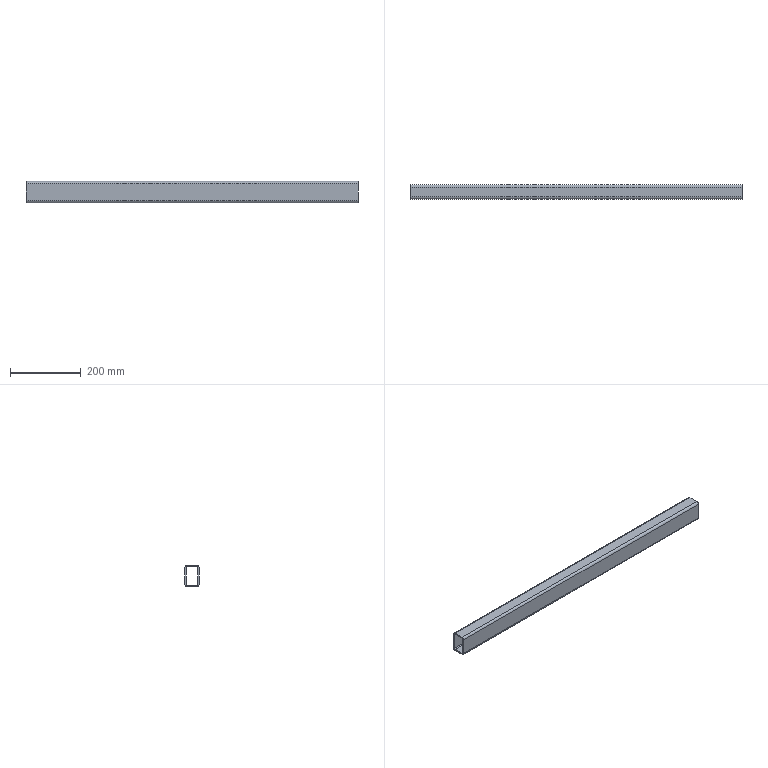Part | STEP file | 40 x 60 x 940_Default<Machined> | 1 solid | 18 faces | box 940 x 40 x 60 mm | volume 663437 mm3 | plane 10 | cylinder 8 | commonest cylinder face diameters 4.8 x4 12.8 x4
STEP:
#1=CARTESIAN_POINT('',(-587.922,20.,23.6));
#2=VERTEX_POINT('',#1);
#3=CARTESIAN_POINT('',(-587.922,13.6,30.));
#4=VERTEX_POINT('',#3);
#5=CARTESIAN_POINT('',(-587.922,13.6,23.6));
#6=DIRECTION('',(1.,0.,0.));
#7=DIRECTION('',(0.,0.,-1.));
#8=AXIS2_PLACEMENT_3D('',#5,#6,#7);
#9=CIRCLE('',#8,6.4);
#10=EDGE_CURVE('',#2,#4,#9,.T.);
#11=ORIENTED_EDGE('',*,*,#10,.T.);
#12=CARTESIAN_POINT('',(352.078,13.6,30.));
#13=VERTEX_POINT('',#12);
#14=CARTESIAN_POINT('',(352.078,13.6,30.));
#15=DIRECTION('',(-1.,0.,0.));
#16=VECTOR('',#15,1000.);
#17=LINE('',#14,#16);
#18=EDGE_CURVE('',#13,#4,#17,.T.);
#19=ORIENTED_EDGE('',*,*,#18,.F.);
#20=CARTESIAN_POINT('',(352.078,20.,23.6));
#21=VERTEX_POINT('',#20);
#22=CARTESIAN_POINT('',(352.078,13.6,23.6));
#23=DIRECTION('',(1.,0.,0.));
#24=DIRECTION('',(0.,0.,-1.));
#25=AXIS2_PLACEMENT_3D('',#22,#23,#24);
#26=CIRCLE('',#25,6.4);
#27=EDGE_CURVE('',#21,#13,#26,.T.);
#28=ORIENTED_EDGE('',*,*,#27,.F.);
#29=CARTESIAN_POINT('',(352.078,20.,23.6));
#30=DIRECTION('',(-1.,0.,0.));
#31=VECTOR('',#30,1000.);
#32=LINE('',#29,#31);
#33=EDGE_CURVE('',#21,#2,#32,.T.);
#34=ORIENTED_EDGE('',*,*,#33,.T.);
#35=EDGE_LOOP('',(#11,#19,#28,#34));
#36=FACE_OUTER_BOUND('',#35,.T.);
#37=CARTESIAN_POINT('',(352.078,13.6,23.6));
#38=DIRECTION('',(-1.,0.,0.));
#39=DIRECTION('',(0.,0.,1.));
#40=AXIS2_PLACEMENT_3D('',#37,#38,#39);
#41=CYLINDRICAL_SURFACE('',#40,6.4);
#42=ADVANCED_FACE('',(#36),#41,.T.);
#43=CARTESIAN_POINT('',(-587.922,-13.6,30.));
#44=VERTEX_POINT('',#43);
#45=CARTESIAN_POINT('',(-587.922,13.6,30.));
#46=DIRECTION('',(0.,-1.,0.));
#47=VECTOR('',#46,1000.);
#48=LINE('',#45,#47);
#49=EDGE_CURVE('',#4,#44,#48,.T.);
#50=ORIENTED_EDGE('',*,*,#49,.T.);
#51=CARTESIAN_POINT('',(352.078,-13.6,30.));
#52=VERTEX_POINT('',#51);
#53=CARTESIAN_POINT('',(352.078,-13.6,30.));
#54=DIRECTION('',(-1.,0.,0.));
#55=VECTOR('',#54,1000.);
#56=LINE('',#53,#55);
#57=EDGE_CURVE('',#52,#44,#56,.T.);
#58=ORIENTED_EDGE('',*,*,#57,.F.);
#59=CARTESIAN_POINT('',(352.078,13.6,30.));
#60=DIRECTION('',(0.,-1.,0.));
#61=VECTOR('',#60,1000.);
#62=LINE('',#59,#61);
#63=EDGE_CURVE('',#13,#52,#62,.T.);
#64=ORIENTED_EDGE('',*,*,#63,.F.);
#65=ORIENTED_EDGE('',*,*,#18,.T.);
#66=EDGE_LOOP('',(#50,#58,#64,#65));
#67=FACE_OUTER_BOUND('',#66,.T.);
#68=CARTESIAN_POINT('',(352.078,13.6,30.));
#69=DIRECTION('',(0.,0.,-1.));
#70=DIRECTION('',(-1.,0.,0.));
#71=AXIS2_PLACEMENT_3D('',#68,#69,#70);
#72=PLANE('',#71);
#73=ADVANCED_FACE('',(#67),#72,.F.);
#74=CARTESIAN_POINT('',(-587.922,-20.,23.6));
#75=VERTEX_POINT('',#74);
#76=CARTESIAN_POINT('',(-587.922,-13.6,23.6));
#77=DIRECTION('',(1.,0.,0.));
#78=DIRECTION('',(0.,0.,-1.));
#79=AXIS2_PLACEMENT_3D('',#76,#77,#78);
#80=CIRCLE('',#79,6.4);
#81=EDGE_CURVE('',#44,#75,#80,.T.);
#82=ORIENTED_EDGE('',*,*,#81,.T.);
#83=CARTESIAN_POINT('',(352.078,-20.,23.6));
#84=VERTEX_POINT('',#83);
#85=CARTESIAN_POINT('',(352.078,-20.,23.6));
#86=DIRECTION('',(-1.,0.,0.));
#87=VECTOR('',#86,1000.);
#88=LINE('',#85,#87);
#89=EDGE_CURVE('',#84,#75,#88,.T.);
#90=ORIENTED_EDGE('',*,*,#89,.F.);
#91=CARTESIAN_POINT('',(352.078,-13.6,23.6));
#92=DIRECTION('',(1.,0.,0.));
#93=DIRECTION('',(0.,0.,-1.));
#94=AXIS2_PLACEMENT_3D('',#91,#92,#93);
#95=CIRCLE('',#94,6.4);
#96=EDGE_CURVE('',#52,#84,#95,.T.);
#97=ORIENTED_EDGE('',*,*,#96,.F.);
#98=ORIENTED_EDGE('',*,*,#57,.T.);
#99=EDGE_LOOP('',(#82,#90,#97,#98));
#100=FACE_OUTER_BOUND('',#99,.T.);
#101=CARTESIAN_POINT('',(352.078,-13.6,23.6));
#102=DIRECTION('',(-1.,0.,0.));
#103=DIRECTION('',(0.,0.,1.));
#104=AXIS2_PLACEMENT_3D('',#101,#102,#103);
#105=CYLINDRICAL_SURFACE('',#104,6.4);
#106=ADVANCED_FACE('',(#100),#105,.T.);
#107=CARTESIAN_POINT('',(-587.922,-20.,-23.6));
#108=VERTEX_POINT('',#107);
#109=CARTESIAN_POINT('',(-587.922,-20.,-23.6));
#110=DIRECTION('',(0.,0.,-1.));
#111=VECTOR('',#110,1000.);
#112=LINE('',#109,#111);
#113=EDGE_CURVE('',#75,#108,#112,.T.);
#114=ORIENTED_EDGE('',*,*,#113,.T.);
#115=CARTESIAN_POINT('',(352.078,-20.,-23.6));
#116=VERTEX_POINT('',#115);
#117=CARTESIAN_POINT('',(352.078,-20.,-23.6));
#118=DIRECTION('',(-1.,0.,0.));
#119=VECTOR('',#118,1000.);
#120=LINE('',#117,#119);
#121=EDGE_CURVE('',#116,#108,#120,.T.);
#122=ORIENTED_EDGE('',*,*,#121,.F.);
#123=CARTESIAN_POINT('',(352.078,-20.,-23.6));
#124=DIRECTION('',(0.,0.,-1.));
#125=VECTOR('',#124,1000.);
#126=LINE('',#123,#125);
#127=EDGE_CURVE('',#84,#116,#126,.T.);
#128=ORIENTED_EDGE('',*,*,#127,.F.);
#129=ORIENTED_EDGE('',*,*,#89,.T.);
#130=EDGE_LOOP('',(#114,#122,#128,#129));
#131=FACE_OUTER_BOUND('',#130,.T.);
#132=CARTESIAN_POINT('',(352.078,-20.,-23.6));
#133=DIRECTION('',(0.,1.,0.));
#134=DIRECTION('',(0.,0.,1.));
#135=AXIS2_PLACEMENT_3D('',#132,#133,#134);
#136=PLANE('',#135);
#137=ADVANCED_FACE('',(#131),#136,.F.);
#138=CARTESIAN_POINT('',(-587.922,-13.6,-30.));
#139=VERTEX_POINT('',#138);
#140=CARTESIAN_POINT('',(-587.922,-13.6,-23.6));
#141=DIRECTION('',(1.,0.,0.));
#142=DIRECTION('',(0.,0.,-1.));
#143=AXIS2_PLACEMENT_3D('',#140,#141,#142);
#144=CIRCLE('',#143,6.4);
#145=EDGE_CURVE('',#108,#139,#144,.T.);
#146=ORIENTED_EDGE('',*,*,#145,.T.);
#147=CARTESIAN_POINT('',(352.078,-13.6,-30.));
#148=VERTEX_POINT('',#147);
#149=CARTESIAN_POINT('',(352.078,-13.6,-30.));
#150=DIRECTION('',(-1.,0.,0.));
#151=VECTOR('',#150,1000.);
#152=LINE('',#149,#151);
#153=EDGE_CURVE('',#148,#139,#152,.T.);
#154=ORIENTED_EDGE('',*,*,#153,.F.);
#155=CARTESIAN_POINT('',(352.078,-13.6,-23.6));
#156=DIRECTION('',(1.,0.,0.));
#157=DIRECTION('',(0.,0.,-1.));
#158=AXIS2_PLACEMENT_3D('',#155,#156,#157);
#159=CIRCLE('',#158,6.4);
#160=EDGE_CURVE('',#116,#148,#159,.T.);
#161=ORIENTED_EDGE('',*,*,#160,.F.);
#162=ORIENTED_EDGE('',*,*,#121,.T.);
#163=EDGE_LOOP('',(#146,#154,#161,#162));
#164=FACE_OUTER_BOUND('',#163,.T.);
#165=CARTESIAN_POINT('',(352.078,-13.6,-23.6));
#166=DIRECTION('',(-1.,0.,0.));
#167=DIRECTION('',(0.,0.,1.));
#168=AXIS2_PLACEMENT_3D('',#165,#166,#167);
#169=CYLINDRICAL_SURFACE('',#168,6.4);
#170=ADVANCED_FACE('',(#164),#169,.T.);
#171=CARTESIAN_POINT('',(-587.922,13.6,-30.));
#172=VERTEX_POINT('',#171);
#173=CARTESIAN_POINT('',(-587.922,-13.6,-30.));
#174=DIRECTION('',(0.,1.,0.));
#175=VECTOR('',#174,1000.);
#176=LINE('',#173,#175);
#177=EDGE_CURVE('',#139,#172,#176,.T.);
#178=ORIENTED_EDGE('',*,*,#177,.T.);
#179=CARTESIAN_POINT('',(352.078,13.6,-30.));
#180=VERTEX_POINT('',#179);
#181=CARTESIAN_POINT('',(352.078,13.6,-30.));
#182=DIRECTION('',(-1.,0.,0.));
#183=VECTOR('',#182,1000.);
#184=LINE('',#181,#183);
#185=EDGE_CURVE('',#180,#172,#184,.T.);
#186=ORIENTED_EDGE('',*,*,#185,.F.);
#187=CARTESIAN_POINT('',(352.078,-13.6,-30.));
#188=DIRECTION('',(0.,1.,0.));
#189=VECTOR('',#188,1000.);
#190=LINE('',#187,#189);
#191=EDGE_CURVE('',#148,#180,#190,.T.);
#192=ORIENTED_EDGE('',*,*,#191,.F.);
#193=ORIENTED_EDGE('',*,*,#153,.T.);
#194=EDGE_LOOP('',(#178,#186,#192,#193));
#195=FACE_OUTER_BOUND('',#194,.T.);
#196=CARTESIAN_POINT('',(352.078,-13.6,-30.));
#197=DIRECTION('',(0.,0.,1.));
#198=DIRECTION('',(1.,0.,0.));
#199=AXIS2_PLACEMENT_3D('',#196,#197,#198);
#200=PLANE('',#199);
#201=ADVANCED_FACE('',(#195),#200,.F.);
#202=CARTESIAN_POINT('',(-587.922,20.,-23.6));
#203=VERTEX_POINT('',#202);
#204=CARTESIAN_POINT('',(-587.922,13.6,-23.6));
#205=DIRECTION('',(1.,0.,0.));
#206=DIRECTION('',(0.,0.,-1.));
#207=AXIS2_PLACEMENT_3D('',#204,#205,#206);
#208=CIRCLE('',#207,6.4);
#209=EDGE_CURVE('',#172,#203,#208,.T.);
#210=ORIENTED_EDGE('',*,*,#209,.T.);
#211=CARTESIAN_POINT('',(352.078,20.,-23.6));
#212=VERTEX_POINT('',#211);
#213=CARTESIAN_POINT('',(352.078,20.,-23.6));
#214=DIRECTION('',(-1.,0.,0.));
#215=VECTOR('',#214,1000.);
#216=LINE('',#213,#215);
#217=EDGE_CURVE('',#212,#203,#216,.T.);
#218=ORIENTED_EDGE('',*,*,#217,.F.);
#219=CARTESIAN_POINT('',(352.078,13.6,-23.6));
#220=DIRECTION('',(1.,0.,0.));
#221=DIRECTION('',(0.,0.,-1.));
#222=AXIS2_PLACEMENT_3D('',#219,#220,#221);
#223=CIRCLE('',#222,6.4);
#224=EDGE_CURVE('',#180,#212,#223,.T.);
#225=ORIENTED_EDGE('',*,*,#224,.F.);
#226=ORIENTED_EDGE('',*,*,#185,.T.);
#227=EDGE_LOOP('',(#210,#218,#225,#226));
#228=FACE_OUTER_BOUND('',#227,.T.);
#229=CARTESIAN_POINT('',(352.078,13.6,-23.6));
#230=DIRECTION('',(-1.,0.,0.));
#231=DIRECTION('',(0.,0.,1.));
#232=AXIS2_PLACEMENT_3D('',#229,#230,#231);
#233=CYLINDRICAL_SURFACE('',#232,6.4);
#234=ADVANCED_FACE('',(#228),#233,.T.);
#235=CARTESIAN_POINT('',(-587.922,-13.6,26.));
#236=VERTEX_POINT('',#235);
#237=CARTESIAN_POINT('',(-587.922,-16.,23.6));
#238=VERTEX_POINT('',#237);
#239=CARTESIAN_POINT('',(-587.922,-13.6,23.6));
#240=DIRECTION('',(1.,0.,0.));
#241=DIRECTION('',(0.,0.,-1.));
#242=AXIS2_PLACEMENT_3D('',#239,#240,#241);
#243=CIRCLE('',#242,2.4);
#244=EDGE_CURVE('',#236,#238,#243,.T.);
#245=ORIENTED_EDGE('',*,*,#244,.F.);
#246=CARTESIAN_POINT('',(352.078,-13.6,26.));
#247=VERTEX_POINT('',#246);
#248=CARTESIAN_POINT('',(352.078,-13.6,26.));
#249=DIRECTION('',(-1.,0.,0.));
#250=VECTOR('',#249,1000.);
#251=LINE('',#248,#250);
#252=EDGE_CURVE('',#247,#236,#251,.T.);
#253=ORIENTED_EDGE('',*,*,#252,.F.);
#254=CARTESIAN_POINT('',(352.078,-16.,23.6));
#255=VERTEX_POINT('',#254);
#256=CARTESIAN_POINT('',(352.078,-13.6,23.6));
#257=DIRECTION('',(1.,0.,0.));
#258=DIRECTION('',(0.,0.,-1.));
#259=AXIS2_PLACEMENT_3D('',#256,#257,#258);
#260=CIRCLE('',#259,2.4);
#261=EDGE_CURVE('',#247,#255,#260,.T.);
#262=ORIENTED_EDGE('',*,*,#261,.T.);
#263=CARTESIAN_POINT('',(352.078,-16.,23.6));
#264=DIRECTION('',(-1.,0.,0.));
#265=VECTOR('',#264,1000.);
#266=LINE('',#263,#265);
#267=EDGE_CURVE('',#255,#238,#266,.T.);
#268=ORIENTED_EDGE('',*,*,#267,.T.);
#269=EDGE_LOOP('',(#245,#253,#262,#268));
#270=FACE_OUTER_BOUND('',#269,.T.);
#271=CARTESIAN_POINT('',(352.078,-13.6,23.6));
#272=DIRECTION('',(-1.,0.,0.));
#273=DIRECTION('',(0.,0.,1.));
#274=AXIS2_PLACEMENT_3D('',#271,#272,#273);
#275=CYLINDRICAL_SURFACE('',#274,2.4);
#276=ADVANCED_FACE('',(#270),#275,.F.);
#277=CARTESIAN_POINT('',(-587.922,13.6,26.));
#278=VERTEX_POINT('',#277);
#279=CARTESIAN_POINT('',(-587.922,13.6,26.));
#280=DIRECTION('',(0.,-1.,0.));
#281=VECTOR('',#280,1000.);
#282=LINE('',#279,#281);
#283=EDGE_CURVE('',#278,#236,#282,.T.);
#284=ORIENTED_EDGE('',*,*,#283,.F.);
#285=CARTESIAN_POINT('',(352.078,13.6,26.));
#286=VERTEX_POINT('',#285);
#287=CARTESIAN_POINT('',(352.078,13.6,26.));
#288=DIRECTION('',(-1.,0.,0.));
#289=VECTOR('',#288,1000.);
#290=LINE('',#287,#289);
#291=EDGE_CURVE('',#286,#278,#290,.T.);
#292=ORIENTED_EDGE('',*,*,#291,.F.);
#293=CARTESIAN_POINT('',(352.078,13.6,26.));
#294=DIRECTION('',(0.,-1.,0.));
#295=VECTOR('',#294,1000.);
#296=LINE('',#293,#295);
#297=EDGE_CURVE('',#286,#247,#296,.T.);
#298=ORIENTED_EDGE('',*,*,#297,.T.);
#299=ORIENTED_EDGE('',*,*,#252,.T.);
#300=EDGE_LOOP('',(#284,#292,#298,#299));
#301=FACE_OUTER_BOUND('',#300,.T.);
#302=CARTESIAN_POINT('',(352.078,13.6,26.));
#303=DIRECTION('',(0.,0.,-1.));
#304=DIRECTION('',(-1.,0.,0.));
#305=AXIS2_PLACEMENT_3D('',#302,#303,#304);
#306=PLANE('',#305);
#307=ADVANCED_FACE('',(#301),#306,.T.);
#308=CARTESIAN_POINT('',(-587.922,16.,23.6));
#309=VERTEX_POINT('',#308);
#310=CARTESIAN_POINT('',(-587.922,13.6,23.6));
#311=DIRECTION('',(1.,0.,0.));
#312=DIRECTION('',(0.,0.,-1.));
#313=AXIS2_PLACEMENT_3D('',#310,#311,#312);
#314=CIRCLE('',#313,2.4);
#315=EDGE_CURVE('',#309,#278,#314,.T.);
#316=ORIENTED_EDGE('',*,*,#315,.F.);
#317=CARTESIAN_POINT('',(352.078,16.,23.6));
#318=VERTEX_POINT('',#317);
#319=CARTESIAN_POINT('',(352.078,16.,23.6));
#320=DIRECTION('',(-1.,0.,0.));
#321=VECTOR('',#320,1000.);
#322=LINE('',#319,#321);
#323=EDGE_CURVE('',#318,#309,#322,.T.);
#324=ORIENTED_EDGE('',*,*,#323,.F.);
#325=CARTESIAN_POINT('',(352.078,13.6,23.6));
#326=DIRECTION('',(1.,0.,0.));
#327=DIRECTION('',(0.,0.,-1.));
#328=AXIS2_PLACEMENT_3D('',#325,#326,#327);
#329=CIRCLE('',#328,2.4);
#330=EDGE_CURVE('',#318,#286,#329,.T.);
#331=ORIENTED_EDGE('',*,*,#330,.T.);
#332=ORIENTED_EDGE('',*,*,#291,.T.);
#333=EDGE_LOOP('',(#316,#324,#331,#332));
#334=FACE_OUTER_BOUND('',#333,.T.);
#335=CARTESIAN_POINT('',(352.078,13.6,23.6));
#336=DIRECTION('',(-1.,0.,0.));
#337=DIRECTION('',(0.,0.,1.));
#338=AXIS2_PLACEMENT_3D('',#335,#336,#337);
#339=CYLINDRICAL_SURFACE('',#338,2.4);
#340=ADVANCED_FACE('',(#334),#339,.F.);
#341=CARTESIAN_POINT('',(-587.922,16.,-23.6));
#342=VERTEX_POINT('',#341);
#343=CARTESIAN_POINT('',(-587.922,16.,23.6));
#344=DIRECTION('',(0.,0.,1.));
#345=VECTOR('',#344,1000.);
#346=LINE('',#343,#345);
#347=EDGE_CURVE('',#342,#309,#346,.T.);
#348=ORIENTED_EDGE('',*,*,#347,.F.);
#349=CARTESIAN_POINT('',(352.078,16.,-23.6));
#350=VERTEX_POINT('',#349);
#351=CARTESIAN_POINT('',(352.078,16.,-23.6));
#352=DIRECTION('',(-1.,0.,0.));
#353=VECTOR('',#352,1000.);
#354=LINE('',#351,#353);
#355=EDGE_CURVE('',#350,#342,#354,.T.);
#356=ORIENTED_EDGE('',*,*,#355,.F.);
#357=CARTESIAN_POINT('',(352.078,16.,23.6));
#358=DIRECTION('',(0.,0.,1.));
#359=VECTOR('',#358,1000.);
#360=LINE('',#357,#359);
#361=EDGE_CURVE('',#350,#318,#360,.T.);
#362=ORIENTED_EDGE('',*,*,#361,.T.);
#363=ORIENTED_EDGE('',*,*,#323,.T.);
#364=EDGE_LOOP('',(#348,#356,#362,#363));
#365=FACE_OUTER_BOUND('',#364,.T.);
#366=CARTESIAN_POINT('',(352.078,16.,23.6));
#367=DIRECTION('',(0.,-1.,0.));
#368=DIRECTION('',(0.,0.,-1.));
#369=AXIS2_PLACEMENT_3D('',#366,#367,#368);
#370=PLANE('',#369);
#371=ADVANCED_FACE('',(#365),#370,.T.);
#372=CARTESIAN_POINT('',(-587.922,13.6,-26.));
#373=VERTEX_POINT('',#372);
#374=CARTESIAN_POINT('',(-587.922,13.6,-23.6));
#375=DIRECTION('',(1.,0.,0.));
#376=DIRECTION('',(0.,0.,-1.));
#377=AXIS2_PLACEMENT_3D('',#374,#375,#376);
#378=CIRCLE('',#377,2.4);
#379=EDGE_CURVE('',#373,#342,#378,.T.);
#380=ORIENTED_EDGE('',*,*,#379,.F.);
#381=CARTESIAN_POINT('',(352.078,13.6,-26.));
#382=VERTEX_POINT('',#381);
#383=CARTESIAN_POINT('',(352.078,13.6,-26.));
#384=DIRECTION('',(-1.,0.,0.));
#385=VECTOR('',#384,1000.);
#386=LINE('',#383,#385);
#387=EDGE_CURVE('',#382,#373,#386,.T.);
#388=ORIENTED_EDGE('',*,*,#387,.F.);
#389=CARTESIAN_POINT('',(352.078,13.6,-23.6));
#390=DIRECTION('',(1.,0.,0.));
#391=DIRECTION('',(0.,0.,-1.));
#392=AXIS2_PLACEMENT_3D('',#389,#390,#391);
#393=CIRCLE('',#392,2.4);
#394=EDGE_CURVE('',#382,#350,#393,.T.);
#395=ORIENTED_EDGE('',*,*,#394,.T.);
#396=ORIENTED_EDGE('',*,*,#355,.T.);
#397=EDGE_LOOP('',(#380,#388,#395,#396));
#398=FACE_OUTER_BOUND('',#397,.T.);
#399=CARTESIAN_POINT('',(352.078,13.6,-23.6));
#400=DIRECTION('',(-1.,0.,0.));
#401=DIRECTION('',(0.,0.,1.));
#402=AXIS2_PLACEMENT_3D('',#399,#400,#401);
#403=CYLINDRICAL_SURFACE('',#402,2.4);
#404=ADVANCED_FACE('',(#398),#403,.F.);
#405=CARTESIAN_POINT('',(-587.922,-13.6,-26.));
#406=VERTEX_POINT('',#405);
#407=CARTESIAN_POINT('',(-587.922,-13.6,-26.));
#408=DIRECTION('',(0.,1.,0.));
#409=VECTOR('',#408,1000.);
#410=LINE('',#407,#409);
#411=EDGE_CURVE('',#406,#373,#410,.T.);
#412=ORIENTED_EDGE('',*,*,#411,.F.);
#413=CARTESIAN_POINT('',(352.078,-13.6,-26.));
#414=VERTEX_POINT('',#413);
#415=CARTESIAN_POINT('',(352.078,-13.6,-26.));
#416=DIRECTION('',(-1.,0.,0.));
#417=VECTOR('',#416,1000.);
#418=LINE('',#415,#417);
#419=EDGE_CURVE('',#414,#406,#418,.T.);
#420=ORIENTED_EDGE('',*,*,#419,.F.);
#421=CARTESIAN_POINT('',(352.078,-13.6,-26.));
#422=DIRECTION('',(0.,1.,0.));
#423=VECTOR('',#422,1000.);
#424=LINE('',#421,#423);
#425=EDGE_CURVE('',#414,#382,#424,.T.);
#426=ORIENTED_EDGE('',*,*,#425,.T.);
#427=ORIENTED_EDGE('',*,*,#387,.T.);
#428=EDGE_LOOP('',(#412,#420,#426,#427));
#429=FACE_OUTER_BOUND('',#428,.T.);
#430=CARTESIAN_POINT('',(352.078,-13.6,-26.));
#431=DIRECTION('',(0.,0.,1.));
#432=DIRECTION('',(1.,0.,0.));
#433=AXIS2_PLACEMENT_3D('',#430,#431,#432);
#434=PLANE('',#433);
#435=ADVANCED_FACE('',(#429),#434,.T.);
#436=CARTESIAN_POINT('',(-587.922,-16.,-23.6));
#437=VERTEX_POINT('',#436);
#438=CARTESIAN_POINT('',(-587.922,-13.6,-23.6));
#439=DIRECTION('',(1.,0.,0.));
#440=DIRECTION('',(0.,0.,-1.));
#441=AXIS2_PLACEMENT_3D('',#438,#439,#440);
#442=CIRCLE('',#441,2.4);
#443=EDGE_CURVE('',#437,#406,#442,.T.);
#444=ORIENTED_EDGE('',*,*,#443,.F.);
#445=CARTESIAN_POINT('',(352.078,-16.,-23.6));
#446=VERTEX_POINT('',#445);
#447=CARTESIAN_POINT('',(352.078,-16.,-23.6));
#448=DIRECTION('',(-1.,0.,0.));
#449=VECTOR('',#448,1000.);
#450=LINE('',#447,#449);
#451=EDGE_CURVE('',#446,#437,#450,.T.);
#452=ORIENTED_EDGE('',*,*,#451,.F.);
#453=CARTESIAN_POINT('',(352.078,-13.6,-23.6));
#454=DIRECTION('',(1.,0.,0.));
#455=DIRECTION('',(0.,0.,-1.));
#456=AXIS2_PLACEMENT_3D('',#453,#454,#455);
#457=CIRCLE('',#456,2.4);
#458=EDGE_CURVE('',#446,#414,#457,.T.);
#459=ORIENTED_EDGE('',*,*,#458,.T.);
#460=ORIENTED_EDGE('',*,*,#419,.T.);
#461=EDGE_LOOP('',(#444,#452,#459,#460));
#462=FACE_OUTER_BOUND('',#461,.T.);
#463=CARTESIAN_POINT('',(352.078,-13.6,-23.6));
#464=DIRECTION('',(-1.,0.,0.));
#465=DIRECTION('',(0.,0.,1.));
#466=AXIS2_PLACEMENT_3D('',#463,#464,#465);
#467=CYLINDRICAL_SURFACE('',#466,2.4);
#468=ADVANCED_FACE('',(#462),#467,.F.);
#469=CARTESIAN_POINT('',(-587.922,-16.,-23.6));
#470=DIRECTION('',(0.,0.,-1.));
#471=VECTOR('',#470,1000.);
#472=LINE('',#469,#471);
#473=EDGE_CURVE('',#238,#437,#472,.T.);
#474=ORIENTED_EDGE('',*,*,#473,.F.);
#475=ORIENTED_EDGE('',*,*,#267,.F.);
#476=CARTESIAN_POINT('',(352.078,-16.,-23.6));
#477=DIRECTION('',(0.,0.,-1.));
#478=VECTOR('',#477,1000.);
#479=LINE('',#476,#478);
#480=EDGE_CURVE('',#255,#446,#479,.T.);
#481=ORIENTED_EDGE('',*,*,#480,.T.);
#482=ORIENTED_EDGE('',*,*,#451,.T.);
#483=EDGE_LOOP('',(#474,#475,#481,#482));
#484=FACE_OUTER_BOUND('',#483,.T.);
#485=CARTESIAN_POINT('',(352.078,-16.,-23.6));
#486=DIRECTION('',(0.,1.,0.));
#487=DIRECTION('',(0.,0.,1.));
#488=AXIS2_PLACEMENT_3D('',#485,#486,#487);
#489=PLANE('',#488);
#490=ADVANCED_FACE('',(#484),#489,.T.);
#491=CARTESIAN_POINT('',(-587.922,20.,23.6));
#492=DIRECTION('',(0.,0.,1.));
#493=VECTOR('',#492,1000.);
#494=LINE('',#491,#493);
#495=EDGE_CURVE('',#203,#2,#494,.T.);
#496=ORIENTED_EDGE('',*,*,#495,.T.);
#497=ORIENTED_EDGE('',*,*,#33,.F.);
#498=CARTESIAN_POINT('',(352.078,20.,23.6));
#499=DIRECTION('',(0.,0.,1.));
#500=VECTOR('',#499,1000.);
#501=LINE('',#498,#500);
#502=EDGE_CURVE('',#212,#21,#501,.T.);
#503=ORIENTED_EDGE('',*,*,#502,.F.);
#504=ORIENTED_EDGE('',*,*,#217,.T.);
#505=EDGE_LOOP('',(#496,#497,#503,#504));
#506=FACE_OUTER_BOUND('',#505,.T.);
#507=CARTESIAN_POINT('',(352.078,20.,23.6));
#508=DIRECTION('',(0.,-1.,0.));
#509=DIRECTION('',(0.,0.,-1.));
#510=AXIS2_PLACEMENT_3D('',#507,#508,#509);
#511=PLANE('',#510);
#512=ADVANCED_FACE('',(#506),#511,.F.);
#513=ORIENTED_EDGE('',*,*,#261,.F.);
#514=ORIENTED_EDGE('',*,*,#297,.F.);
#515=ORIENTED_EDGE('',*,*,#330,.F.);
#516=ORIENTED_EDGE('',*,*,#361,.F.);
#517=ORIENTED_EDGE('',*,*,#394,.F.);
#518=ORIENTED_EDGE('',*,*,#425,.F.);
#519=ORIENTED_EDGE('',*,*,#458,.F.);
#520=ORIENTED_EDGE('',*,*,#480,.F.);
#521=EDGE_LOOP('',(#513,#514,#515,#516,#517,#518,#519,#520));
#522=FACE_BOUND('',#521,.T.);
#523=ORIENTED_EDGE('',*,*,#27,.T.);
#524=ORIENTED_EDGE('',*,*,#63,.T.);
#525=ORIENTED_EDGE('',*,*,#96,.T.);
#526=ORIENTED_EDGE('',*,*,#127,.T.);
#527=ORIENTED_EDGE('',*,*,#160,.T.);
#528=ORIENTED_EDGE('',*,*,#191,.T.);
#529=ORIENTED_EDGE('',*,*,#224,.T.);
#530=ORIENTED_EDGE('',*,*,#502,.T.);
#531=EDGE_LOOP('',(#523,#524,#525,#526,#527,#528,#529,#530));
#532=FACE_OUTER_BOUND('',#531,.T.);
#533=CARTESIAN_POINT('',(352.078,13.6,23.6));
#534=DIRECTION('',(1.,0.,0.));
#535=DIRECTION('',(0.,0.,-1.));
#536=AXIS2_PLACEMENT_3D('',#533,#534,#535);
#537=PLANE('',#536);
#538=ADVANCED_FACE('',(#522,#532),#537,.T.);
#539=ORIENTED_EDGE('',*,*,#244,.T.);
#540=ORIENTED_EDGE('',*,*,#473,.T.);
#541=ORIENTED_EDGE('',*,*,#443,.T.);
#542=ORIENTED_EDGE('',*,*,#411,.T.);
#543=ORIENTED_EDGE('',*,*,#379,.T.);
#544=ORIENTED_EDGE('',*,*,#347,.T.);
#545=ORIENTED_EDGE('',*,*,#315,.T.);
#546=ORIENTED_EDGE('',*,*,#283,.T.);
#547=EDGE_LOOP('',(#539,#540,#541,#542,#543,#544,#545,#546));
#548=FACE_BOUND('',#547,.T.);
#549=ORIENTED_EDGE('',*,*,#10,.F.);
#550=ORIENTED_EDGE('',*,*,#495,.F.);
#551=ORIENTED_EDGE('',*,*,#209,.F.);
#552=ORIENTED_EDGE('',*,*,#177,.F.);
#553=ORIENTED_EDGE('',*,*,#145,.F.);
#554=ORIENTED_EDGE('',*,*,#113,.F.);
#555=ORIENTED_EDGE('',*,*,#81,.F.);
#556=ORIENTED_EDGE('',*,*,#49,.F.);
#557=EDGE_LOOP('',(#549,#550,#551,#552,#553,#554,#555,#556));
#558=FACE_OUTER_BOUND('',#557,.T.);
#559=CARTESIAN_POINT('',(-587.922,13.6,23.6));
#560=DIRECTION('',(1.,0.,0.));
#561=DIRECTION('',(0.,0.,-1.));
#562=AXIS2_PLACEMENT_3D('',#559,#560,#561);
#563=PLANE('',#562);
#564=ADVANCED_FACE('',(#548,#558),#563,.F.);
#565=CLOSED_SHELL('',(#42,#73,#106,#137,#170,#201,#234,#276,#307,#340,#371,#404,#435,#468,#490,#512,#538,#564));
#566=MANIFOLD_SOLID_BREP('',#565);
#567=CARTESIAN_POINT('',(0.,0.,0.));
#568=DIRECTION('',(0.,0.,1.));
#569=DIRECTION('',(1.,0.,0.));
#570=AXIS2_PLACEMENT_3D('',#567,#568,#569);
#571=(LENGTH_UNIT()NAMED_UNIT(*)SI_UNIT(.MILLI.,.METRE.));
#572=UNCERTAINTY_MEASURE_WITH_UNIT(LENGTH_MEASURE(0.00001),#571,'','');
#573=(NAMED_UNIT(*)PLANE_ANGLE_UNIT()SI_UNIT($,.RADIAN.));
#574=(NAMED_UNIT(*)SI_UNIT($,.STERADIAN.)SOLID_ANGLE_UNIT());
#575=(GEOMETRIC_REPRESENTATION_CONTEXT(3)GLOBAL_UNCERTAINTY_ASSIGNED_CONTEXT((#572))GLOBAL_UNIT_ASSIGNED_CONTEXT((#571,#573,#574))REPRESENTATION_CONTEXT('',''));
#576=ADVANCED_BREP_SHAPE_REPRESENTATION('',(#566,#570),#575);